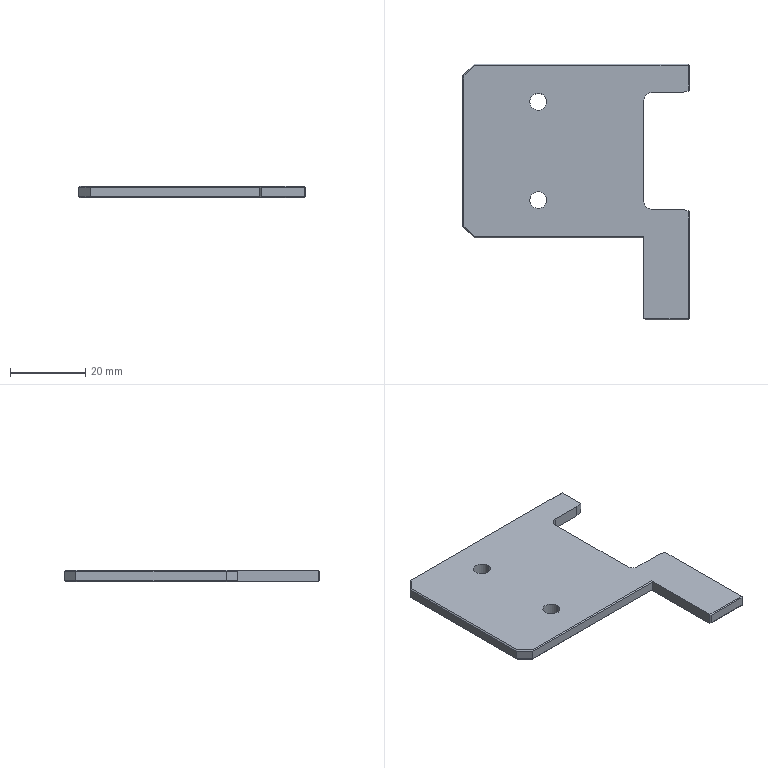Part | STEP file | Riveting station pick claw | 1 solid | 47 faces | box 60 x 67.74 x 3 mm | volume 7814 mm3 | plane 41 | cylinder 6 | commonest cylinder face diameters 4.5 x4 4 x2